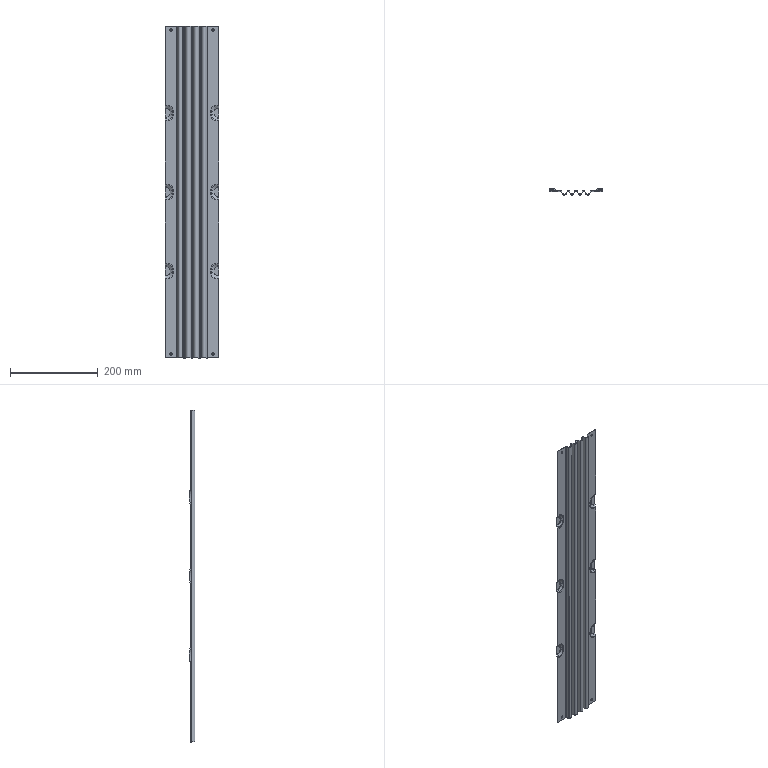Part | NX | features BREP 1 | 1 solid | 254 faces | box 122 x 13.6 x 755.2 mm | volume 141700 mm3 | cylinder 104 | plane 78 | torus 48 | cone 24 | commonest cylinder face diameters 2 x18 3.6 x18 4.4 x18 6 x18 1 x8 3.4 x8